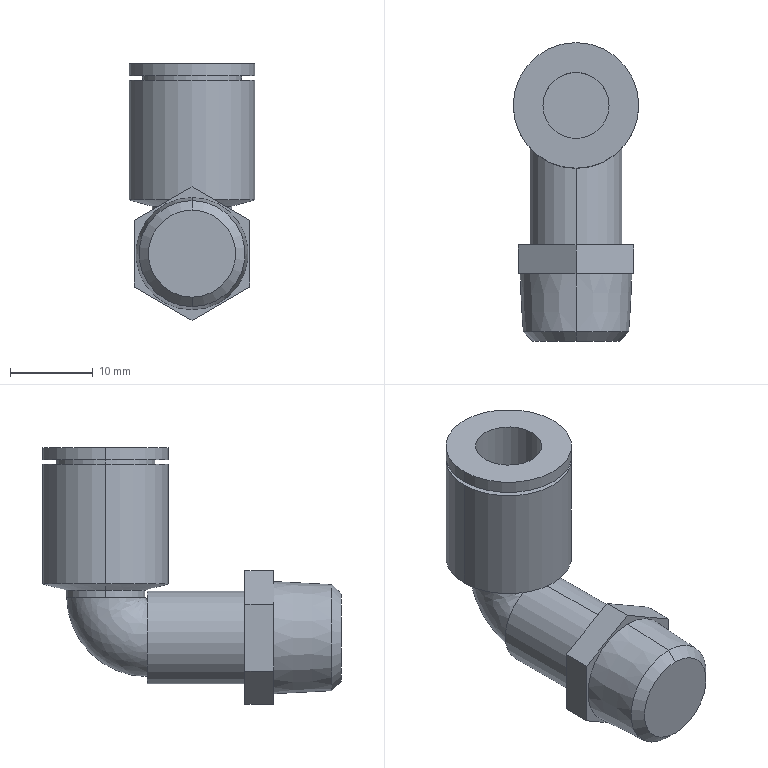Part | SolidWorks | features BaseBody 1 | 1 solid | 35 faces | box 15.2 x 36.1 x 31.083 mm | volume 5569 mm3 | plane 15 | cylinder 12 | cone 6 | spline 2 | commonest cylinder face diameters 15.2 x4 8 x2 9.637 x2 11.2 x2 12 x2
STEP:
#1=CARTESIAN_POINT('',(-7.6,28.5,21.));
#2=VERTEX_POINT('',#1);
#3=CARTESIAN_POINT('',(7.6,28.5,21.));
#4=VERTEX_POINT('',#3);
#5=CARTESIAN_POINT('',(0.,28.5,21.));
#6=DIRECTION('',(0.,0.,-1.));
#7=DIRECTION('',(-1.,0.,0.));
#8=AXIS2_PLACEMENT_3D('',#5,#6,#7);
#9=CIRCLE('',#8,7.6);
#10=EDGE_CURVE('',#2,#4,#9,.T.);
#11=ORIENTED_EDGE('',*,*,#10,.T.);
#12=CARTESIAN_POINT('',(7.6,28.5,6.495));
#13=VERTEX_POINT('',#12);
#14=CARTESIAN_POINT('',(7.6,28.5,13.748));
#15=DIRECTION('',(0.,0.,-1.));
#16=VECTOR('',#15,1000.);
#17=LINE('',#14,#16);
#18=EDGE_CURVE('',#4,#13,#17,.T.);
#19=ORIENTED_EDGE('',*,*,#18,.T.);
#20=CARTESIAN_POINT('',(-7.6,28.5,6.495));
#21=VERTEX_POINT('',#20);
#22=CARTESIAN_POINT('',(0.,28.5,6.495));
#23=DIRECTION('',(0.,0.,1.));
#24=DIRECTION('',(-1.,0.,0.));
#25=AXIS2_PLACEMENT_3D('',#22,#23,#24);
#26=CIRCLE('',#25,7.6);
#27=EDGE_CURVE('',#13,#21,#26,.T.);
#28=ORIENTED_EDGE('',*,*,#27,.T.);
#29=CARTESIAN_POINT('',(-7.6,28.5,13.748));
#30=DIRECTION('',(0.,0.,-1.));
#31=VECTOR('',#30,1000.);
#32=LINE('',#29,#31);
#33=EDGE_CURVE('',#2,#21,#32,.T.);
#34=ORIENTED_EDGE('',*,*,#33,.F.);
#35=EDGE_LOOP('',(#11,#19,#28,#34));
#36=FACE_OUTER_BOUND('',#35,.T.);
#37=CARTESIAN_POINT('',(0.,28.5,13.748));
#38=DIRECTION('',(0.,0.,-1.));
#39=DIRECTION('',(-1.,0.,0.));
#40=AXIS2_PLACEMENT_3D('',#37,#38,#39);
#41=CYLINDRICAL_SURFACE('',#40,7.6);
#42=ADVANCED_FACE('',(#36),#41,.T.);
#43=CARTESIAN_POINT('',(4.818,28.5,5.75));
#44=VERTEX_POINT('',#43);
#45=CARTESIAN_POINT('',(-4.818,28.5,5.75));
#46=VERTEX_POINT('',#45);
#47=CARTESIAN_POINT('',(0.,28.5,5.75));
#48=DIRECTION('',(0.,0.,1.));
#49=DIRECTION('',(-1.,0.,0.));
#50=AXIS2_PLACEMENT_3D('',#47,#48,#49);
#51=CIRCLE('',#50,4.818);
#52=EDGE_CURVE('',#44,#46,#51,.T.);
#53=ORIENTED_EDGE('',*,*,#52,.T.);
#54=CARTESIAN_POINT('',(-7.6,28.5,6.495));
#55=DIRECTION('',(-0.9659,0.,0.2588));
#56=VECTOR('',#55,1000.);
#57=LINE('',#54,#56);
#58=EDGE_CURVE('',#46,#21,#57,.T.);
#59=ORIENTED_EDGE('',*,*,#58,.T.);
#60=ORIENTED_EDGE('',*,*,#27,.F.);
#61=CARTESIAN_POINT('',(7.6,28.5,6.495));
#62=DIRECTION('',(0.9659,0.,0.2588));
#63=VECTOR('',#62,1000.);
#64=LINE('',#61,#63);
#65=EDGE_CURVE('',#44,#13,#64,.T.);
#66=ORIENTED_EDGE('',*,*,#65,.F.);
#67=EDGE_LOOP('',(#53,#59,#60,#66));
#68=FACE_OUTER_BOUND('',#67,.T.);
#69=CARTESIAN_POINT('',(0.,28.5,6.495));
#70=DIRECTION('',(0.,0.,1.));
#71=DIRECTION('',(1.,0.,0.));
#72=AXIS2_PLACEMENT_3D('',#69,#70,#71);
#73=CONICAL_SURFACE('',#72,7.6,1.309);
#74=ADVANCED_FACE('',(#68),#73,.T.);
#75=ORIENTED_EDGE('',*,*,#52,.F.);
#76=CARTESIAN_POINT('',(4.818,28.5,4.864));
#77=VERTEX_POINT('',#76);
#78=CARTESIAN_POINT('',(4.818,28.5,5.307));
#79=DIRECTION('',(0.,0.,-1.));
#80=VECTOR('',#79,1000.);
#81=LINE('',#78,#80);
#82=EDGE_CURVE('',#44,#77,#81,.T.);
#83=ORIENTED_EDGE('',*,*,#82,.T.);
#84=CARTESIAN_POINT('',(-4.818,28.5,4.864));
#85=VERTEX_POINT('',#84);
#86=CARTESIAN_POINT('',(0.,28.5,4.864));
#87=DIRECTION('',(0.,0.,1.));
#88=DIRECTION('',(-1.,0.,0.));
#89=AXIS2_PLACEMENT_3D('',#86,#87,#88);
#90=CIRCLE('',#89,4.818);
#91=EDGE_CURVE('',#77,#85,#90,.T.);
#92=ORIENTED_EDGE('',*,*,#91,.T.);
#93=CARTESIAN_POINT('',(-4.818,28.5,5.307));
#94=DIRECTION('',(0.,0.,-1.));
#95=VECTOR('',#94,1000.);
#96=LINE('',#93,#95);
#97=EDGE_CURVE('',#46,#85,#96,.T.);
#98=ORIENTED_EDGE('',*,*,#97,.F.);
#99=EDGE_LOOP('',(#75,#83,#92,#98));
#100=FACE_OUTER_BOUND('',#99,.T.);
#101=CARTESIAN_POINT('',(0.,28.5,5.307));
#102=DIRECTION('',(0.,0.,-1.));
#103=DIRECTION('',(-1.,0.,0.));
#104=AXIS2_PLACEMENT_3D('',#101,#102,#103);
#105=CYLINDRICAL_SURFACE('',#104,4.818);
#106=ADVANCED_FACE('',(#100),#105,.T.);
#107=CARTESIAN_POINT('',(-6.,28.5,21.5));
#108=VERTEX_POINT('',#107);
#109=CARTESIAN_POINT('',(6.,28.5,21.5));
#110=VERTEX_POINT('',#109);
#111=CARTESIAN_POINT('',(0.,28.5,21.5));
#112=DIRECTION('',(0.,0.,-1.));
#113=DIRECTION('',(-1.,0.,0.));
#114=AXIS2_PLACEMENT_3D('',#111,#112,#113);
#115=CIRCLE('',#114,6.);
#116=EDGE_CURVE('',#108,#110,#115,.T.);
#117=ORIENTED_EDGE('',*,*,#116,.T.);
#118=CARTESIAN_POINT('',(6.,28.5,21.));
#119=VERTEX_POINT('',#118);
#120=CARTESIAN_POINT('',(6.,28.5,21.25));
#121=DIRECTION('',(0.,0.,-1.));
#122=VECTOR('',#121,1000.);
#123=LINE('',#120,#122);
#124=EDGE_CURVE('',#110,#119,#123,.T.);
#125=ORIENTED_EDGE('',*,*,#124,.T.);
#126=CARTESIAN_POINT('',(-6.,28.5,21.));
#127=VERTEX_POINT('',#126);
#128=CARTESIAN_POINT('',(0.,28.5,21.));
#129=DIRECTION('',(0.,0.,-1.));
#130=DIRECTION('',(-1.,0.,0.));
#131=AXIS2_PLACEMENT_3D('',#128,#129,#130);
#132=CIRCLE('',#131,6.);
#133=EDGE_CURVE('',#127,#119,#132,.T.);
#134=ORIENTED_EDGE('',*,*,#133,.F.);
#135=CARTESIAN_POINT('',(-6.,28.5,21.25));
#136=DIRECTION('',(0.,0.,-1.));
#137=VECTOR('',#136,1000.);
#138=LINE('',#135,#137);
#139=EDGE_CURVE('',#108,#127,#138,.T.);
#140=ORIENTED_EDGE('',*,*,#139,.F.);
#141=EDGE_LOOP('',(#117,#125,#134,#140));
#142=FACE_OUTER_BOUND('',#141,.T.);
#143=CARTESIAN_POINT('',(0.,28.5,21.25));
#144=DIRECTION('',(0.,0.,-1.));
#145=DIRECTION('',(-1.,0.,0.));
#146=AXIS2_PLACEMENT_3D('',#143,#144,#145);
#147=CYLINDRICAL_SURFACE('',#146,6.);
#148=ADVANCED_FACE('',(#142),#147,.T.);
#149=CARTESIAN_POINT('',(0.,23.747,4.864));
#150=VERTEX_POINT('',#149);
#151=CARTESIAN_POINT('',(0.,33.211,4.864));
#152=VERTEX_POINT('',#151);
#153=CARTESIAN_POINT('',(0.,23.747,4.864));
#154=CARTESIAN_POINT('',(0.3117,23.747,4.864));
#155=CARTESIAN_POINT('',(0.6231,23.784,4.864));
#156=CARTESIAN_POINT('',(1.226,23.915,4.864));
#157=CARTESIAN_POINT('',(1.519,24.008,4.864));
#158=CARTESIAN_POINT('',(2.087,24.25,4.864));
#159=CARTESIAN_POINT('',(2.362,24.399,4.864));
#160=CARTESIAN_POINT('',(2.872,24.743,4.864));
#161=CARTESIAN_POINT('',(3.109,24.938,4.864));
#162=CARTESIAN_POINT('',(3.547,25.377,4.864));
#163=CARTESIAN_POINT('',(3.744,25.618,4.864));
#164=CARTESIAN_POINT('',(4.086,26.128,4.864));
#165=CARTESIAN_POINT('',(4.232,26.401,4.864));
#166=CARTESIAN_POINT('',(4.47,26.975,4.864));
#167=CARTESIAN_POINT('',(4.56,27.269,4.864));
#168=CARTESIAN_POINT('',(4.68,27.872,4.864));
#169=CARTESIAN_POINT('',(4.712,28.184,4.864));
#170=CARTESIAN_POINT('',(4.712,28.801,4.864));
#171=CARTESIAN_POINT('',(4.683,29.107,4.864));
#172=CARTESIAN_POINT('',(4.563,29.712,4.864));
#173=CARTESIAN_POINT('',(4.473,30.012,4.864));
#174=CARTESIAN_POINT('',(4.238,30.581,4.864));
#175=CARTESIAN_POINT('',(4.094,30.852,4.864));
#176=CARTESIAN_POINT('',(3.749,31.369,4.864));
#177=CARTESIAN_POINT('',(3.553,31.609,4.864));
#178=CARTESIAN_POINT('',(3.119,32.044,4.864));
#179=CARTESIAN_POINT('',(2.878,32.242,4.864));
#180=CARTESIAN_POINT('',(2.364,32.587,4.864));
#181=CARTESIAN_POINT('',(2.093,32.732,4.864));
#182=CARTESIAN_POINT('',(1.524,32.968,4.864));
#183=CARTESIAN_POINT('',(1.224,33.059,4.864));
#184=CARTESIAN_POINT('',(0.6186,33.18,4.864));
#185=CARTESIAN_POINT('',(0.3115,33.211,4.864));
#186=CARTESIAN_POINT('',(0.,33.211,4.864));
#187=B_SPLINE_CURVE_WITH_KNOTS('',3,(#153,#154,#155,#156,#157,#158,#159,#160,#161,#162,#163,#164,#165,#166,#167,#168,#169,#170,#171,#172,#173,#174,#175,#176,#177,#178,#179,#180,#181,#182,#183,#184,#185,#186),.UNSPECIFIED.,.F.,.F.,(4,2,2,2,2,2,2,2,2,2,2,2,2,2,2,2,4),(0.01474,0.01567,0.01659,0.01751,0.01843,0.01935,0.02027,0.02119,0.02211,0.02303,0.02396,0.02488,0.0258,0.02672,0.02764,0.02856,0.02948),.UNSPECIFIED.);
#188=EDGE_CURVE('',#150,#152,#187,.T.);
#189=ORIENTED_EDGE('',*,*,#188,.F.);
#190=CARTESIAN_POINT('',(0.,23.484,4.712));
#191=VERTEX_POINT('',#190);
#192=CARTESIAN_POINT('',(0.,23.484,5.016));
#193=DIRECTION('',(-1.,0.,0.));
#194=DIRECTION('',(0.,0.,1.));
#195=AXIS2_PLACEMENT_3D('',#192,#193,#194);
#196=CIRCLE('',#195,0.304);
#197=EDGE_CURVE('',#150,#191,#196,.T.);
#198=ORIENTED_EDGE('',*,*,#197,.T.);
#199=CARTESIAN_POINT('',(0.,23.484,-4.712));
#200=VERTEX_POINT('',#199);
#201=CARTESIAN_POINT('',(0.,23.484,4.712));
#202=CARTESIAN_POINT('',(0.3112,23.484,4.712));
#203=CARTESIAN_POINT('',(0.6228,23.484,4.681));
#204=CARTESIAN_POINT('',(1.227,23.484,4.56));
#205=CARTESIAN_POINT('',(1.521,23.484,4.47));
#206=CARTESIAN_POINT('',(2.09,23.484,4.234));
#207=CARTESIAN_POINT('',(2.366,23.484,4.086));
#208=CARTESIAN_POINT('',(2.877,23.484,3.744));
#209=CARTESIAN_POINT('',(3.114,23.484,3.55));
#210=CARTESIAN_POINT('',(3.553,23.484,3.111));
#211=CARTESIAN_POINT('',(3.749,23.484,2.871));
#212=CARTESIAN_POINT('',(4.09,23.484,2.361));
#213=CARTESIAN_POINT('',(4.236,23.484,2.086));
#214=CARTESIAN_POINT('',(4.473,23.484,1.514));
#215=CARTESIAN_POINT('',(4.562,23.484,1.22));
#216=CARTESIAN_POINT('',(4.682,23.484,0.617));
#217=CARTESIAN_POINT('',(4.712,23.484,0.3048));
#218=CARTESIAN_POINT('',(4.712,23.484,-0.3105));
#219=CARTESIAN_POINT('',(4.682,23.484,-0.6159));
#220=CARTESIAN_POINT('',(4.561,23.484,-1.222));
#221=CARTESIAN_POINT('',(4.47,23.484,-1.521));
#222=CARTESIAN_POINT('',(4.235,23.484,-2.088));
#223=CARTESIAN_POINT('',(4.09,23.484,-2.36));
#224=CARTESIAN_POINT('',(3.745,23.484,-2.877));
#225=CARTESIAN_POINT('',(3.55,23.484,-3.114));
#226=CARTESIAN_POINT('',(3.116,23.484,-3.548));
#227=CARTESIAN_POINT('',(2.874,23.484,-3.747));
#228=CARTESIAN_POINT('',(2.361,23.484,-4.09));
#229=CARTESIAN_POINT('',(2.09,23.484,-4.234));
#230=CARTESIAN_POINT('',(1.521,23.484,-4.47));
#231=CARTESIAN_POINT('',(1.221,23.484,-4.561));
#232=CARTESIAN_POINT('',(0.6176,23.484,-4.681));
#233=CARTESIAN_POINT('',(0.3112,23.484,-4.712));
#234=CARTESIAN_POINT('',(0.,23.484,-4.712));
#235=B_SPLINE_CURVE_WITH_KNOTS('',3,(#201,#202,#203,#204,#205,#206,#207,#208,#209,#210,#211,#212,#213,#214,#215,#216,#217,#218,#219,#220,#221,#222,#223,#224,#225,#226,#227,#228,#229,#230,#231,#232,#233,#234),.UNSPECIFIED.,.F.,.F.,(4,2,2,2,2,2,2,2,2,2,2,2,2,2,2,2,4),(0.007389,0.008313,0.009237,0.01016,0.01109,0.01201,0.01293,0.01386,0.01478,0.01571,0.01663,0.01755,0.01848,0.0194,0.02033,0.02125,0.02217),.UNSPECIFIED.);
#236=EDGE_CURVE('',#191,#200,#235,.T.);
#237=ORIENTED_EDGE('',*,*,#236,.T.);
#238=CARTESIAN_POINT('',(0.,23.484,5.016));
#239=DIRECTION('',(-1.,0.,0.));
#240=DIRECTION('',(0.,0.,1.));
#241=AXIS2_PLACEMENT_3D('',#238,#239,#240);
#242=CIRCLE('',#241,9.728);
#243=EDGE_CURVE('',#152,#200,#242,.T.);
#244=ORIENTED_EDGE('',*,*,#243,.F.);
#245=EDGE_LOOP('',(#189,#198,#237,#244));
#246=FACE_OUTER_BOUND('',#245,.T.);
#247=CARTESIAN_POINT('',(0.,33.212,4.955));
#248=CARTESIAN_POINT('',(0.,33.176,-0.7153));
#249=CARTESIAN_POINT('',(0.,29.154,-4.712));
#250=CARTESIAN_POINT('',(0.,23.484,-4.712));
#251=CARTESIAN_POINT('',(9.424,33.212,4.955));
#252=CARTESIAN_POINT('',(9.424,33.176,-0.7153));
#253=CARTESIAN_POINT('',(9.424,29.154,-4.712));
#254=CARTESIAN_POINT('',(9.424,23.484,-4.712));
#255=CARTESIAN_POINT('',(9.424,23.788,5.014));
#256=CARTESIAN_POINT('',(9.424,23.787,4.837));
#257=CARTESIAN_POINT('',(9.424,23.661,4.712));
#258=CARTESIAN_POINT('',(9.424,23.484,4.712));
#259=CARTESIAN_POINT('',(0.,23.788,5.014));
#260=CARTESIAN_POINT('',(0.,23.787,4.837));
#261=CARTESIAN_POINT('',(0.,23.661,4.712));
#262=CARTESIAN_POINT('',(0.,23.484,4.712));
#263=(BOUNDED_SURFACE()B_SPLINE_SURFACE(3,3,((#247,#248,#249,#250),(#251,#252,#253,#254),(#255,#256,#257,#258),(#259,#260,#261,#262)),.UNSPECIFIED.,.F.,.F.,.F.)B_SPLINE_SURFACE_WITH_KNOTS((4,4),(4,4),(0.,1.),(0.,1.),.UNSPECIFIED.)GEOMETRIC_REPRESENTATION_ITEM()RATIONAL_B_SPLINE_SURFACE(((1.,0.8062,0.8062,1.),(0.3333,0.2687,0.2687,0.3333),(0.3333,0.2687,0.2687,0.3333),(1.,0.8062,0.8062,1.)))REPRESENTATION_ITEM('')SURFACE());
#264=ADVANCED_FACE('',(#246),#263,.T.);
#265=CARTESIAN_POINT('',(-7.6,28.5,23.));
#266=VERTEX_POINT('',#265);
#267=CARTESIAN_POINT('',(7.6,28.5,23.));
#268=VERTEX_POINT('',#267);
#269=CARTESIAN_POINT('',(0.,28.5,23.));
#270=DIRECTION('',(0.,0.,-1.));
#271=DIRECTION('',(-1.,0.,0.));
#272=AXIS2_PLACEMENT_3D('',#269,#270,#271);
#273=CIRCLE('',#272,7.6);
#274=EDGE_CURVE('',#266,#268,#273,.T.);
#275=ORIENTED_EDGE('',*,*,#274,.T.);
#276=CARTESIAN_POINT('',(7.6,28.5,21.5));
#277=VERTEX_POINT('',#276);
#278=CARTESIAN_POINT('',(7.6,28.5,22.25));
#279=DIRECTION('',(0.,0.,-1.));
#280=VECTOR('',#279,1000.);
#281=LINE('',#278,#280);
#282=EDGE_CURVE('',#268,#277,#281,.T.);
#283=ORIENTED_EDGE('',*,*,#282,.T.);
#284=CARTESIAN_POINT('',(-7.6,28.5,21.5));
#285=VERTEX_POINT('',#284);
#286=CARTESIAN_POINT('',(0.,28.5,21.5));
#287=DIRECTION('',(0.,0.,-1.));
#288=DIRECTION('',(-1.,0.,0.));
#289=AXIS2_PLACEMENT_3D('',#286,#287,#288);
#290=CIRCLE('',#289,7.6);
#291=EDGE_CURVE('',#285,#277,#290,.T.);
#292=ORIENTED_EDGE('',*,*,#291,.F.);
#293=CARTESIAN_POINT('',(-7.6,28.5,22.25));
#294=DIRECTION('',(0.,0.,-1.));
#295=VECTOR('',#294,1000.);
#296=LINE('',#293,#295);
#297=EDGE_CURVE('',#266,#285,#296,.T.);
#298=ORIENTED_EDGE('',*,*,#297,.F.);
#299=EDGE_LOOP('',(#275,#283,#292,#298));
#300=FACE_OUTER_BOUND('',#299,.T.);
#301=CARTESIAN_POINT('',(0.,28.5,22.25));
#302=DIRECTION('',(0.,0.,-1.));
#303=DIRECTION('',(-1.,0.,0.));
#304=AXIS2_PLACEMENT_3D('',#301,#302,#303);
#305=CYLINDRICAL_SURFACE('',#304,7.6);
#306=ADVANCED_FACE('',(#300),#305,.T.);
#307=CARTESIAN_POINT('',(0.,11.66,5.6));
#308=VERTEX_POINT('',#307);
#309=CARTESIAN_POINT('',(0.,11.66,-5.6));
#310=VERTEX_POINT('',#309);
#311=CARTESIAN_POINT('',(0.,11.66,0.));
#312=DIRECTION('',(0.,1.,0.));
#313=DIRECTION('',(0.,0.,1.));
#314=AXIS2_PLACEMENT_3D('',#311,#312,#313);
#315=CIRCLE('',#314,5.6);
#316=EDGE_CURVE('',#308,#310,#315,.T.);
#317=ORIENTED_EDGE('',*,*,#316,.T.);
#318=CARTESIAN_POINT('',(0.,23.484,-5.6));
#319=VERTEX_POINT('',#318);
#320=CARTESIAN_POINT('',(0.,15.958,-5.6));
#321=DIRECTION('',(0.,1.,0.));
#322=VECTOR('',#321,1000.);
#323=LINE('',#320,#322);
#324=EDGE_CURVE('',#310,#319,#323,.T.);
#325=ORIENTED_EDGE('',*,*,#324,.T.);
#326=CARTESIAN_POINT('',(0.,23.484,5.6));
#327=VERTEX_POINT('',#326);
#328=CARTESIAN_POINT('',(0.,23.484,0.));
#329=DIRECTION('',(0.,1.,0.));
#330=DIRECTION('',(0.,0.,1.));
#331=AXIS2_PLACEMENT_3D('',#328,#329,#330);
#332=CIRCLE('',#331,5.6);
#333=EDGE_CURVE('',#327,#319,#332,.T.);
#334=ORIENTED_EDGE('',*,*,#333,.F.);
#335=CARTESIAN_POINT('',(0.,15.958,5.6));
#336=DIRECTION('',(0.,1.,0.));
#337=VECTOR('',#336,1000.);
#338=LINE('',#335,#337);
#339=EDGE_CURVE('',#308,#327,#338,.T.);
#340=ORIENTED_EDGE('',*,*,#339,.F.);
#341=EDGE_LOOP('',(#317,#325,#334,#340));
#342=FACE_OUTER_BOUND('',#341,.T.);
#343=CARTESIAN_POINT('',(0.,15.958,0.));
#344=DIRECTION('',(0.,1.,0.));
#345=DIRECTION('',(0.,0.,1.));
#346=AXIS2_PLACEMENT_3D('',#343,#344,#345);
#347=CYLINDRICAL_SURFACE('',#346,5.6);
#348=ADVANCED_FACE('',(#342),#347,.T.);
#349=CARTESIAN_POINT('',(-4.,28.5,4.5));
#350=VERTEX_POINT('',#349);
#351=CARTESIAN_POINT('',(4.,28.5,4.5));
#352=VERTEX_POINT('',#351);
#353=CARTESIAN_POINT('',(0.,28.5,4.5));
#354=DIRECTION('',(0.,0.,1.));
#355=DIRECTION('',(1.,0.,0.));
#356=AXIS2_PLACEMENT_3D('',#353,#354,#355);
#357=CIRCLE('',#356,4.);
#358=EDGE_CURVE('',#350,#352,#357,.T.);
#359=ORIENTED_EDGE('',*,*,#358,.F.);
#360=CARTESIAN_POINT('',(-4.,28.5,23.));
#361=VERTEX_POINT('',#360);
#362=CARTESIAN_POINT('',(-4.,28.5,41.5));
#363=DIRECTION('',(0.,0.,1.));
#364=VECTOR('',#363,1000.);
#365=LINE('',#362,#364);
#366=EDGE_CURVE('',#350,#361,#365,.T.);
#367=ORIENTED_EDGE('',*,*,#366,.T.);
#368=CARTESIAN_POINT('',(4.,28.5,23.));
#369=VERTEX_POINT('',#368);
#370=CARTESIAN_POINT('',(0.,28.5,23.));
#371=DIRECTION('',(0.,0.,-1.));
#372=DIRECTION('',(1.,0.,0.));
#373=AXIS2_PLACEMENT_3D('',#370,#371,#372);
#374=CIRCLE('',#373,4.);
#375=EDGE_CURVE('',#369,#361,#374,.T.);
#376=ORIENTED_EDGE('',*,*,#375,.F.);
#377=CARTESIAN_POINT('',(4.,28.5,41.5));
#378=DIRECTION('',(0.,0.,1.));
#379=VECTOR('',#378,1000.);
#380=LINE('',#377,#379);
#381=EDGE_CURVE('',#352,#369,#380,.T.);
#382=ORIENTED_EDGE('',*,*,#381,.F.);
#383=EDGE_LOOP('',(#359,#367,#376,#382));
#384=FACE_OUTER_BOUND('',#383,.T.);
#385=CARTESIAN_POINT('',(0.,28.5,41.5));
#386=DIRECTION('',(0.,0.,1.));
#387=DIRECTION('',(1.,0.,0.));
#388=AXIS2_PLACEMENT_3D('',#385,#386,#387);
#389=CYLINDRICAL_SURFACE('',#388,4.);
#390=ADVANCED_FACE('',(#384),#389,.F.);
#391=CARTESIAN_POINT('',(0.,1.146,6.418));
#392=VERTEX_POINT('',#391);
#393=CARTESIAN_POINT('',(0.,1.146,-6.418));
#394=VERTEX_POINT('',#393);
#395=CARTESIAN_POINT('',(0.,1.146,0.));
#396=DIRECTION('',(0.,1.,0.));
#397=DIRECTION('',(-1.,0.,0.));
#398=AXIS2_PLACEMENT_3D('',#395,#396,#397);
#399=CIRCLE('',#398,6.418);
#400=EDGE_CURVE('',#392,#394,#399,.T.);
#401=ORIENTED_EDGE('',*,*,#400,.T.);
#402=CARTESIAN_POINT('',(0.,8.16,-6.786));
#403=VERTEX_POINT('',#402);
#404=CARTESIAN_POINT('',(0.,8.16,-6.786));
#405=DIRECTION('',(0.,0.9986,-0.05234));
#406=VECTOR('',#405,1000.);
#407=LINE('',#404,#406);
#408=EDGE_CURVE('',#394,#403,#407,.T.);
#409=ORIENTED_EDGE('',*,*,#408,.T.);
#410=CARTESIAN_POINT('',(0.,8.16,6.786));
#411=VERTEX_POINT('',#410);
#412=CARTESIAN_POINT('',(0.,8.16,0.));
#413=DIRECTION('',(0.,-1.,0.));
#414=DIRECTION('',(0.,0.,1.));
#415=AXIS2_PLACEMENT_3D('',#412,#413,#414);
#416=CIRCLE('',#415,6.786);
#417=EDGE_CURVE('',#403,#411,#416,.T.);
#418=ORIENTED_EDGE('',*,*,#417,.T.);
#419=CARTESIAN_POINT('',(0.,8.16,6.786));
#420=DIRECTION('',(0.,0.9986,0.05234));
#421=VECTOR('',#420,1000.);
#422=LINE('',#419,#421);
#423=EDGE_CURVE('',#392,#411,#422,.T.);
#424=ORIENTED_EDGE('',*,*,#423,.F.);
#425=EDGE_LOOP('',(#401,#409,#418,#424));
#426=FACE_OUTER_BOUND('',#425,.T.);
#427=CARTESIAN_POINT('',(0.,8.16,0.));
#428=DIRECTION('',(0.,1.,0.));
#429=DIRECTION('',(0.,0.,1.));
#430=AXIS2_PLACEMENT_3D('',#427,#428,#429);
#431=CONICAL_SURFACE('',#430,6.786,0.05236);
#432=ADVANCED_FACE('',(#426),#431,.T.);
#433=CARTESIAN_POINT('',(0.,0.,5.272));
#434=VERTEX_POINT('',#433);
#435=CARTESIAN_POINT('',(0.,0.,-5.272));
#436=VERTEX_POINT('',#435);
#437=CARTESIAN_POINT('',(0.,0.,0.));
#438=DIRECTION('',(0.,1.,0.));
#439=DIRECTION('',(0.,0.,1.));
#440=AXIS2_PLACEMENT_3D('',#437,#438,#439);
#441=CIRCLE('',#440,5.272);
#442=EDGE_CURVE('',#434,#436,#441,.T.);
#443=ORIENTED_EDGE('',*,*,#442,.T.);
#444=CARTESIAN_POINT('',(0.,1.146,-6.418));
#445=DIRECTION('',(0.,0.7071,-0.7071));
#446=VECTOR('',#445,1000.);
#447=LINE('',#444,#446);
#448=EDGE_CURVE('',#436,#394,#447,.T.);
#449=ORIENTED_EDGE('',*,*,#448,.T.);
#450=ORIENTED_EDGE('',*,*,#400,.F.);
#451=CARTESIAN_POINT('',(0.,1.146,6.418));
#452=DIRECTION('',(0.,0.7071,0.7071));
#453=VECTOR('',#452,1000.);
#454=LINE('',#451,#453);
#455=EDGE_CURVE('',#434,#392,#454,.T.);
#456=ORIENTED_EDGE('',*,*,#455,.F.);
#457=EDGE_LOOP('',(#443,#449,#450,#456));
#458=FACE_OUTER_BOUND('',#457,.T.);
#459=CARTESIAN_POINT('',(0.,1.146,0.));
#460=DIRECTION('',(0.,1.,0.));
#461=DIRECTION('',(0.,0.,1.));
#462=AXIS2_PLACEMENT_3D('',#459,#460,#461);
#463=CONICAL_SURFACE('',#462,6.418,0.7854);
#464=ADVANCED_FACE('',(#458),#463,.T.);
#465=ORIENTED_EDGE('',*,*,#18,.F.);
#466=CARTESIAN_POINT('',(0.,28.5,21.));
#467=DIRECTION('',(0.,0.,-1.));
#468=DIRECTION('',(-1.,0.,0.));
#469=AXIS2_PLACEMENT_3D('',#466,#467,#468);
#470=CIRCLE('',#469,7.6);
#471=EDGE_CURVE('',#4,#2,#470,.T.);
#472=ORIENTED_EDGE('',*,*,#471,.T.);
#473=ORIENTED_EDGE('',*,*,#33,.T.);
#474=CARTESIAN_POINT('',(0.,28.5,6.495));
#475=DIRECTION('',(0.,0.,1.));
#476=DIRECTION('',(-1.,0.,0.));
#477=AXIS2_PLACEMENT_3D('',#474,#475,#476);
#478=CIRCLE('',#477,7.6);
#479=EDGE_CURVE('',#21,#13,#478,.T.);
#480=ORIENTED_EDGE('',*,*,#479,.T.);
#481=EDGE_LOOP('',(#465,#472,#473,#480));
#482=FACE_OUTER_BOUND('',#481,.T.);
#483=CARTESIAN_POINT('',(0.,28.5,13.748));
#484=DIRECTION('',(0.,0.,-1.));
#485=DIRECTION('',(-1.,0.,0.));
#486=AXIS2_PLACEMENT_3D('',#483,#484,#485);
#487=CYLINDRICAL_SURFACE('',#486,7.6);
#488=ADVANCED_FACE('',(#482),#487,.T.);
#489=ORIENTED_EDGE('',*,*,#58,.F.);
#490=CARTESIAN_POINT('',(0.,28.5,5.75));
#491=DIRECTION('',(0.,0.,1.));
#492=DIRECTION('',(-1.,0.,0.));
#493=AXIS2_PLACEMENT_3D('',#490,#491,#492);
#494=CIRCLE('',#493,4.818);
#495=EDGE_CURVE('',#46,#44,#494,.T.);
#496=ORIENTED_EDGE('',*,*,#495,.T.);
#497=ORIENTED_EDGE('',*,*,#65,.T.);
#498=ORIENTED_EDGE('',*,*,#479,.F.);
#499=EDGE_LOOP('',(#489,#496,#497,#498));
#500=FACE_OUTER_BOUND('',#499,.T.);
#501=CARTESIAN_POINT('',(0.,28.5,6.495));
#502=DIRECTION('',(0.,0.,1.));
#503=DIRECTION('',(1.,0.,0.));
#504=AXIS2_PLACEMENT_3D('',#501,#502,#503);
#505=CONICAL_SURFACE('',#504,7.6,1.309);
#506=ADVANCED_FACE('',(#500),#505,.T.);
#507=ORIENTED_EDGE('',*,*,#10,.F.);
#508=ORIENTED_EDGE('',*,*,#471,.F.);
#509=EDGE_LOOP('',(#507,#508));
#510=FACE_OUTER_BOUND('',#509,.T.);
#511=ORIENTED_EDGE('',*,*,#133,.T.);
#512=CARTESIAN_POINT('',(0.,28.5,21.));
#513=DIRECTION('',(0.,0.,-1.));
#514=DIRECTION('',(-1.,0.,0.));
#515=AXIS2_PLACEMENT_3D('',#512,#513,#514);
#516=CIRCLE('',#515,6.);
#517=EDGE_CURVE('',#119,#127,#516,.T.);
#518=ORIENTED_EDGE('',*,*,#517,.T.);
#519=EDGE_LOOP('',(#511,#518));
#520=FACE_BOUND('',#519,.T.);
#521=CARTESIAN_POINT('',(-6.8,28.5,21.));
#522=DIRECTION('',(0.,0.,1.));
#523=DIRECTION('',(1.,0.,0.));
#524=AXIS2_PLACEMENT_3D('',#521,#522,#523);
#525=PLANE('',#524);
#526=ADVANCED_FACE('',(#510,#520),#525,.T.);
#527=ORIENTED_EDGE('',*,*,#82,.F.);
#528=ORIENTED_EDGE('',*,*,#495,.F.);
#529=ORIENTED_EDGE('',*,*,#97,.T.);
#530=CARTESIAN_POINT('',(0.,28.5,4.864));
#531=DIRECTION('',(0.,0.,1.));
#532=DIRECTION('',(-1.,0.,0.));
#533=AXIS2_PLACEMENT_3D('',#530,#531,#532);
#534=CIRCLE('',#533,4.818);
#535=EDGE_CURVE('',#85,#77,#534,.T.);
#536=ORIENTED_EDGE('',*,*,#535,.T.);
#537=EDGE_LOOP('',(#527,#528,#529,#536));
#538=FACE_OUTER_BOUND('',#537,.T.);
#539=CARTESIAN_POINT('',(0.,28.5,5.307));
#540=DIRECTION('',(0.,0.,-1.));
#541=DIRECTION('',(-1.,0.,0.));
#542=AXIS2_PLACEMENT_3D('',#539,#540,#541);
#543=CYLINDRICAL_SURFACE('',#542,4.818);
#544=ADVANCED_FACE('',(#538),#543,.T.);
#545=ORIENTED_EDGE('',*,*,#124,.F.);
#546=CARTESIAN_POINT('',(0.,28.5,21.5));
#547=DIRECTION('',(0.,0.,-1.));
#548=DIRECTION('',(-1.,0.,0.));
#549=AXIS2_PLACEMENT_3D('',#546,#547,#548);
#550=CIRCLE('',#549,6.);
#551=EDGE_CURVE('',#110,#108,#550,.T.);
#552=ORIENTED_EDGE('',*,*,#551,.T.);
#553=ORIENTED_EDGE('',*,*,#139,.T.);
#554=ORIENTED_EDGE('',*,*,#517,.F.);
#555=EDGE_LOOP('',(#545,#552,#553,#554));
#556=FACE_OUTER_BOUND('',#555,.T.);
#557=CARTESIAN_POINT('',(0.,28.5,21.25));
#558=DIRECTION('',(0.,0.,-1.));
#559=DIRECTION('',(-1.,0.,0.));
#560=AXIS2_PLACEMENT_3D('',#557,#558,#559);
#561=CYLINDRICAL_SURFACE('',#560,6.);
#562=ADVANCED_FACE('',(#556),#561,.T.);
#563=CARTESIAN_POINT('',(0.,33.211,4.864));
#564=CARTESIAN_POINT('',(-0.3116,33.211,4.864));
#565=CARTESIAN_POINT('',(-0.618,33.18,4.864));
#566=CARTESIAN_POINT('',(-1.221,33.06,4.864));
#567=CARTESIAN_POINT('',(-1.52,32.97,4.864));
#568=CARTESIAN_POINT('',(-2.091,32.733,4.864));
#569=CARTESIAN_POINT('',(-2.362,32.588,4.864));
#570=CARTESIAN_POINT('',(-2.875,32.245,4.864));
#571=CARTESIAN_POINT('',(-3.117,32.046,4.864));
#572=CARTESIAN_POINT('',(-3.552,31.61,4.864));
#573=CARTESIAN_POINT('',(-3.747,31.372,4.864));
#574=CARTESIAN_POINT('',(-4.091,30.856,4.864));
#575=CARTESIAN_POINT('',(-4.237,30.582,4.864));
#576=CARTESIAN_POINT('',(-4.472,30.014,4.864));
#577=CARTESIAN_POINT('',(-4.562,29.717,4.864));
#578=CARTESIAN_POINT('',(-4.683,29.108,4.864));
#579=CARTESIAN_POINT('',(-4.712,28.802,4.864));
#580=CARTESIAN_POINT('',(-4.712,28.187,4.864));
#581=CARTESIAN_POINT('',(-4.681,27.874,4.864));
#582=CARTESIAN_POINT('',(-4.56,27.27,4.864));
#583=CARTESIAN_POINT('',(-4.47,26.976,4.864));
#584=CARTESIAN_POINT('',(-4.234,26.405,4.864));
#585=CARTESIAN_POINT('',(-4.086,26.129,4.864));
#586=CARTESIAN_POINT('',(-3.744,25.618,4.864));
#587=CARTESIAN_POINT('',(-3.549,25.379,4.864));
#588=CARTESIAN_POINT('',(-3.11,24.938,4.864));
#589=CARTESIAN_POINT('',(-2.871,24.743,4.864));
#590=CARTESIAN_POINT('',(-2.362,24.399,4.864));
#591=CARTESIAN_POINT('',(-2.087,24.25,4.864));
#592=CARTESIAN_POINT('',(-1.518,24.008,4.864));
#593=CARTESIAN_POINT('',(-1.225,23.914,4.864));
#594=CARTESIAN_POINT('',(-0.6232,23.784,4.864));
#595=CARTESIAN_POINT('',(-0.3118,23.747,4.864));
#596=CARTESIAN_POINT('',(0.,23.747,4.864));
#597=B_SPLINE_CURVE_WITH_KNOTS('',3,(#563,#564,#565,#566,#567,#568,#569,#570,#571,#572,#573,#574,#575,#576,#577,#578,#579,#580,#581,#582,#583,#584,#585,#586,#587,#588,#589,#590,#591,#592,#593,#594,#595,#596),.UNSPECIFIED.,.F.,.F.,(4,2,2,2,2,2,2,2,2,2,2,2,2,2,2,2,4),(0.,0.0009215,0.001843,0.002765,0.003686,0.004608,0.005529,0.006451,0.007372,0.008294,0.009215,0.01014,0.01106,0.01198,0.0129,0.01382,0.01474),.UNSPECIFIED.);
#598=EDGE_CURVE('',#152,#150,#597,.T.);
#599=ORIENTED_EDGE('',*,*,#598,.T.);
#600=ORIENTED_EDGE('',*,*,#188,.T.);
#601=EDGE_LOOP('',(#599,#600));
#602=FACE_BOUND('',#601,.T.);
#603=ORIENTED_EDGE('',*,*,#535,.F.);
#604=ORIENTED_EDGE('',*,*,#91,.F.);
#605=EDGE_LOOP('',(#603,#604));
#606=FACE_OUTER_BOUND('',#605,.T.);
#607=CARTESIAN_POINT('',(-2.409,28.5,4.864));
#608=DIRECTION('',(0.,0.,-1.));
#609=DIRECTION('',(-1.,0.,0.));
#610=AXIS2_PLACEMENT_3D('',#607,#608,#609);
#611=PLANE('',#610);
#612=ADVANCED_FACE('',(#602,#606),#611,.T.);
#613=ORIENTED_EDGE('',*,*,#116,.F.);
#614=ORIENTED_EDGE('',*,*,#551,.F.);
#615=EDGE_LOOP('',(#613,#614));
#616=FACE_BOUND('',#615,.T.);
#617=ORIENTED_EDGE('',*,*,#291,.T.);
#618=CARTESIAN_POINT('',(0.,28.5,21.5));
#619=DIRECTION('',(0.,0.,-1.));
#620=DIRECTION('',(-1.,0.,0.));
#621=AXIS2_PLACEMENT_3D('',#618,#619,#620);
#622=CIRCLE('',#621,7.6);
#623=EDGE_CURVE('',#277,#285,#622,.T.);
#624=ORIENTED_EDGE('',*,*,#623,.T.);
#625=EDGE_LOOP('',(#617,#624));
#626=FACE_OUTER_BOUND('',#625,.T.);
#627=CARTESIAN_POINT('',(-6.8,28.5,21.5));
#628=DIRECTION('',(0.,0.,-1.));
#629=DIRECTION('',(-1.,0.,0.));
#630=AXIS2_PLACEMENT_3D('',#627,#628,#629);
#631=PLANE('',#630);
#632=ADVANCED_FACE('',(#616,#626),#631,.T.);
#633=ORIENTED_EDGE('',*,*,#197,.F.);
#634=ORIENTED_EDGE('',*,*,#598,.F.);
#635=ORIENTED_EDGE('',*,*,#243,.T.);
#636=CARTESIAN_POINT('',(0.,23.484,-4.712));
#637=CARTESIAN_POINT('',(-0.3111,23.484,-4.712));
#638=CARTESIAN_POINT('',(-0.617,23.484,-4.681));
#639=CARTESIAN_POINT('',(-1.219,23.484,-4.562));
#640=CARTESIAN_POINT('',(-1.518,23.484,-4.472));
#641=CARTESIAN_POINT('',(-2.088,23.484,-4.235));
#642=CARTESIAN_POINT('',(-2.359,23.484,-4.091));
#643=CARTESIAN_POINT('',(-2.871,23.484,-3.749));
#644=CARTESIAN_POINT('',(-3.113,23.484,-3.551));
#645=CARTESIAN_POINT('',(-3.548,23.484,-3.116));
#646=CARTESIAN_POINT('',(-3.743,23.484,-2.879));
#647=CARTESIAN_POINT('',(-4.087,23.484,-2.365));
#648=CARTESIAN_POINT('',(-4.234,23.484,-2.091));
#649=CARTESIAN_POINT('',(-4.469,23.484,-1.525));
#650=CARTESIAN_POINT('',(-4.56,23.484,-1.228));
#651=CARTESIAN_POINT('',(-4.681,23.484,-0.6199));
#652=CARTESIAN_POINT('',(-4.712,23.484,-0.3122));
#653=CARTESIAN_POINT('',(-4.712,23.484,0.3099));
#654=CARTESIAN_POINT('',(-4.682,23.484,0.6167));
#655=CARTESIAN_POINT('',(-4.561,23.484,1.222));
#656=CARTESIAN_POINT('',(-4.47,23.484,1.521));
#657=CARTESIAN_POINT('',(-4.235,23.484,2.089));
#658=CARTESIAN_POINT('',(-4.09,23.484,2.36));
#659=CARTESIAN_POINT('',(-3.747,23.484,2.874));
#660=CARTESIAN_POINT('',(-3.549,23.484,3.115));
#661=CARTESIAN_POINT('',(-3.116,23.484,3.548));
#662=CARTESIAN_POINT('',(-2.876,23.484,3.745));
#663=CARTESIAN_POINT('',(-2.361,23.484,4.09));
#664=CARTESIAN_POINT('',(-2.09,23.484,4.234));
#665=CARTESIAN_POINT('',(-1.523,23.484,4.47));
#666=CARTESIAN_POINT('',(-1.224,23.484,4.561));
#667=CARTESIAN_POINT('',(-0.618,23.484,4.681));
#668=CARTESIAN_POINT('',(-0.3111,23.484,4.712));
#669=CARTESIAN_POINT('',(0.,23.484,4.712));
#670=B_SPLINE_CURVE_WITH_KNOTS('',3,(#636,#637,#638,#639,#640,#641,#642,#643,#644,#645,#646,#647,#648,#649,#650,#651,#652,#653,#654,#655,#656,#657,#658,#659,#660,#661,#662,#663,#664,#665,#666,#667,#668,#669),.UNSPECIFIED.,.F.,.F.,(4,2,2,2,2,2,2,2,2,2,2,2,2,2,2,2,4),(0.02217,0.0231,0.02402,0.02495,0.02587,0.02679,0.02772,0.02864,0.02956,0.03049,0.03141,0.03234,0.03326,0.03418,0.03511,0.03603,0.03695),.UNSPECIFIED.);
#671=EDGE_CURVE('',#200,#191,#670,.T.);
#672=ORIENTED_EDGE('',*,*,#671,.T.);
#673=EDGE_LOOP('',(#633,#634,#635,#672));
#674=FACE_OUTER_BOUND('',#673,.T.);
#675=CARTESIAN_POINT('',(0.,23.788,5.014));
#676=CARTESIAN_POINT('',(0.,23.787,4.837));
#677=CARTESIAN_POINT('',(0.,23.661,4.712));
#678=CARTESIAN_POINT('',(0.,23.484,4.712));
#679=CARTESIAN_POINT('',(-9.424,23.788,5.014));
#680=CARTESIAN_POINT('',(-9.424,23.787,4.837));
#681=CARTESIAN_POINT('',(-9.424,23.661,4.712));
#682=CARTESIAN_POINT('',(-9.424,23.484,4.712));
#683=CARTESIAN_POINT('',(-9.424,33.212,4.955));
#684=CARTESIAN_POINT('',(-9.424,33.176,-0.7153));
#685=CARTESIAN_POINT('',(-9.424,29.154,-4.712));
#686=CARTESIAN_POINT('',(-9.424,23.484,-4.712));
#687=CARTESIAN_POINT('',(0.,33.212,4.955));
#688=CARTESIAN_POINT('',(0.,33.176,-0.7153));
#689=CARTESIAN_POINT('',(0.,29.154,-4.712));
#690=CARTESIAN_POINT('',(0.,23.484,-4.712));
#691=(BOUNDED_SURFACE()B_SPLINE_SURFACE(3,3,((#675,#676,#677,#678),(#679,#680,#681,#682),(#683,#684,#685,#686),(#687,#688,#689,#690)),.UNSPECIFIED.,.F.,.F.,.F.)B_SPLINE_SURFACE_WITH_KNOTS((4,4),(4,4),(0.,1.),(0.,1.),.UNSPECIFIED.)GEOMETRIC_REPRESENTATION_ITEM()RATIONAL_B_SPLINE_SURFACE(((1.,0.8062,0.8062,1.),(0.3333,0.2687,0.2687,0.3333),(0.3333,0.2687,0.2687,0.3333),(1.,0.8062,0.8062,1.)))REPRESENTATION_ITEM('')SURFACE());
#692=ADVANCED_FACE('',(#674),#691,.T.);
#693=ORIENTED_EDGE('',*,*,#282,.F.);
#694=CARTESIAN_POINT('',(0.,28.5,23.));
#695=DIRECTION('',(0.,0.,-1.));
#696=DIRECTION('',(-1.,0.,0.));
#697=AXIS2_PLACEMENT_3D('',#694,#695,#696);
#698=CIRCLE('',#697,7.6);
#699=EDGE_CURVE('',#268,#266,#698,.T.);
#700=ORIENTED_EDGE('',*,*,#699,.T.);
#701=ORIENTED_EDGE('',*,*,#297,.T.);
#702=ORIENTED_EDGE('',*,*,#623,.F.);
#703=EDGE_LOOP('',(#693,#700,#701,#702));
#704=FACE_OUTER_BOUND('',#703,.T.);
#705=CARTESIAN_POINT('',(0.,28.5,22.25));
#706=DIRECTION('',(0.,0.,-1.));
#707=DIRECTION('',(-1.,0.,0.));
#708=AXIS2_PLACEMENT_3D('',#705,#706,#707);
#709=CYLINDRICAL_SURFACE('',#708,7.6);
#710=ADVANCED_FACE('',(#704),#709,.T.);
#711=ORIENTED_EDGE('',*,*,#333,.T.);
#712=CARTESIAN_POINT('',(0.,23.484,0.));
#713=DIRECTION('',(0.,1.,0.));
#714=DIRECTION('',(0.,0.,1.));
#715=AXIS2_PLACEMENT_3D('',#712,#713,#714);
#716=CIRCLE('',#715,5.6);
#717=EDGE_CURVE('',#319,#327,#716,.T.);
#718=ORIENTED_EDGE('',*,*,#717,.T.);
#719=EDGE_LOOP('',(#711,#718));
#720=FACE_OUTER_BOUND('',#719,.T.);
#721=ORIENTED_EDGE('',*,*,#671,.F.);
#722=ORIENTED_EDGE('',*,*,#236,.F.);
#723=EDGE_LOOP('',(#721,#722));
#724=FACE_BOUND('',#723,.T.);
#725=CARTESIAN_POINT('',(-2.8,23.484,0.));
#726=DIRECTION('',(0.,1.,0.));
#727=DIRECTION('',(0.,0.,1.));
#728=AXIS2_PLACEMENT_3D('',#725,#726,#727);
#729=PLANE('',#728);
#730=ADVANCED_FACE('',(#720,#724),#729,.T.);
#731=ORIENTED_EDGE('',*,*,#274,.F.);
#732=ORIENTED_EDGE('',*,*,#699,.F.);
#733=EDGE_LOOP('',(#731,#732));
#734=FACE_OUTER_BOUND('',#733,.T.);
#735=ORIENTED_EDGE('',*,*,#375,.T.);
#736=CARTESIAN_POINT('',(0.,28.5,23.));
#737=DIRECTION('',(0.,0.,-1.));
#738=DIRECTION('',(1.,0.,0.));
#739=AXIS2_PLACEMENT_3D('',#736,#737,#738);
#740=CIRCLE('',#739,4.);
#741=EDGE_CURVE('',#361,#369,#740,.T.);
#742=ORIENTED_EDGE('',*,*,#741,.T.);
#743=EDGE_LOOP('',(#735,#742));
#744=FACE_BOUND('',#743,.T.);
#745=CARTESIAN_POINT('',(-3.8,28.5,23.));
#746=DIRECTION('',(0.,0.,1.));
#747=DIRECTION('',(1.,0.,0.));
#748=AXIS2_PLACEMENT_3D('',#745,#746,#747);
#749=PLANE('',#748);
#750=ADVANCED_FACE('',(#734,#744),#749,.T.);
#751=ORIENTED_EDGE('',*,*,#324,.F.);
#752=CARTESIAN_POINT('',(0.,11.66,0.));
#753=DIRECTION('',(0.,1.,0.));
#754=DIRECTION('',(0.,0.,1.));
#755=AXIS2_PLACEMENT_3D('',#752,#753,#754);
#756=CIRCLE('',#755,5.6);
#757=EDGE_CURVE('',#310,#308,#756,.T.);
#758=ORIENTED_EDGE('',*,*,#757,.T.);
#759=ORIENTED_EDGE('',*,*,#339,.T.);
#760=ORIENTED_EDGE('',*,*,#717,.F.);
#761=EDGE_LOOP('',(#751,#758,#759,#760));
#762=FACE_OUTER_BOUND('',#761,.T.);
#763=CARTESIAN_POINT('',(0.,15.958,0.));
#764=DIRECTION('',(0.,1.,0.));
#765=DIRECTION('',(0.,0.,1.));
#766=AXIS2_PLACEMENT_3D('',#763,#764,#765);
#767=CYLINDRICAL_SURFACE('',#766,5.6);
#768=ADVANCED_FACE('',(#762),#767,.T.);
#769=ORIENTED_EDGE('',*,*,#366,.F.);
#770=CARTESIAN_POINT('',(0.,28.5,4.5));
#771=DIRECTION('',(0.,0.,1.));
#772=DIRECTION('',(1.,0.,0.));
#773=AXIS2_PLACEMENT_3D('',#770,#771,#772);
#774=CIRCLE('',#773,4.);
#775=EDGE_CURVE('',#352,#350,#774,.T.);
#776=ORIENTED_EDGE('',*,*,#775,.F.);
#777=ORIENTED_EDGE('',*,*,#381,.T.);
#778=ORIENTED_EDGE('',*,*,#741,.F.);
#779=EDGE_LOOP('',(#769,#776,#777,#778));
#780=FACE_OUTER_BOUND('',#779,.T.);
#781=CARTESIAN_POINT('',(0.,28.5,41.5));
#782=DIRECTION('',(0.,0.,1.));
#783=DIRECTION('',(1.,0.,0.));
#784=AXIS2_PLACEMENT_3D('',#781,#782,#783);
#785=CYLINDRICAL_SURFACE('',#784,4.);
#786=ADVANCED_FACE('',(#780),#785,.F.);
#787=ORIENTED_EDGE('',*,*,#316,.F.);
#788=ORIENTED_EDGE('',*,*,#757,.F.);
#789=EDGE_LOOP('',(#787,#788));
#790=FACE_BOUND('',#789,.T.);
#791=CARTESIAN_POINT('',(7.,11.66,4.041));
#792=VERTEX_POINT('',#791);
#793=CARTESIAN_POINT('',(7.,11.66,-4.041));
#794=VERTEX_POINT('',#793);
#795=CARTESIAN_POINT('',(7.,11.66,0.));
#796=DIRECTION('',(0.,0.,-1.));
#797=VECTOR('',#796,1000.);
#798=LINE('',#795,#797);
#799=EDGE_CURVE('',#792,#794,#798,.T.);
#800=ORIENTED_EDGE('',*,*,#799,.T.);
#801=CARTESIAN_POINT('',(0.,11.66,-8.083));
#802=VERTEX_POINT('',#801);
#803=CARTESIAN_POINT('',(7.,11.66,-4.041));
#804=DIRECTION('',(-0.866,0.,-0.5));
#805=VECTOR('',#804,1000.);
#806=LINE('',#803,#805);
#807=EDGE_CURVE('',#794,#802,#806,.T.);
#808=ORIENTED_EDGE('',*,*,#807,.T.);
#809=CARTESIAN_POINT('',(-7.,11.66,-4.041));
#810=VERTEX_POINT('',#809);
#811=CARTESIAN_POINT('',(0.,11.66,-8.083));
#812=DIRECTION('',(-0.866,0.,0.5));
#813=VECTOR('',#812,1000.);
#814=LINE('',#811,#813);
#815=EDGE_CURVE('',#802,#810,#814,.T.);
#816=ORIENTED_EDGE('',*,*,#815,.T.);
#817=CARTESIAN_POINT('',(-7.,11.66,4.041));
#818=VERTEX_POINT('',#817);
#819=CARTESIAN_POINT('',(-7.,11.66,0.));
#820=DIRECTION('',(0.,0.,1.));
#821=VECTOR('',#820,1000.);
#822=LINE('',#819,#821);
#823=EDGE_CURVE('',#810,#818,#822,.T.);
#824=ORIENTED_EDGE('',*,*,#823,.T.);
#825=CARTESIAN_POINT('',(0.,11.66,8.083));
#826=VERTEX_POINT('',#825);
#827=CARTESIAN_POINT('',(-7.,11.66,4.041));
#828=DIRECTION('',(0.866,0.,0.5));
#829=VECTOR('',#828,1000.);
#830=LINE('',#827,#829);
#831=EDGE_CURVE('',#818,#826,#830,.T.);
#832=ORIENTED_EDGE('',*,*,#831,.T.);
#833=CARTESIAN_POINT('',(0.,11.66,8.083));
#834=DIRECTION('',(0.866,0.,-0.5));
#835=VECTOR('',#834,1000.);
#836=LINE('',#833,#835);
#837=EDGE_CURVE('',#826,#792,#836,.T.);
#838=ORIENTED_EDGE('',*,*,#837,.T.);
#839=EDGE_LOOP('',(#800,#808,#816,#824,#832,#838));
#840=FACE_OUTER_BOUND('',#839,.T.);
#841=CARTESIAN_POINT('',(0.,11.66,0.));
#842=DIRECTION('',(0.,1.,0.));
#843=DIRECTION('',(0.,0.,1.));
#844=AXIS2_PLACEMENT_3D('',#841,#842,#843);
#845=PLANE('',#844);
#846=ADVANCED_FACE('',(#790,#840),#845,.T.);
#847=ORIENTED_EDGE('',*,*,#775,.T.);
#848=ORIENTED_EDGE('',*,*,#358,.T.);
#849=EDGE_LOOP('',(#847,#848));
#850=FACE_OUTER_BOUND('',#849,.T.);
#851=CARTESIAN_POINT('',(0.,28.5,4.5));
#852=DIRECTION('',(0.,0.,1.));
#853=DIRECTION('',(1.,0.,0.));
#854=AXIS2_PLACEMENT_3D('',#851,#852,#853);
#855=PLANE('',#854);
#856=ADVANCED_FACE('',(#850),#855,.T.);
#857=CARTESIAN_POINT('',(7.,8.16,-4.041));
#858=VERTEX_POINT('',#857);
#859=CARTESIAN_POINT('',(0.,8.16,-8.083));
#860=VERTEX_POINT('',#859);
#861=CARTESIAN_POINT('',(0.,8.16,-8.083));
#862=DIRECTION('',(-0.866,0.,-0.5));
#863=VECTOR('',#862,1000.);
#864=LINE('',#861,#863);
#865=EDGE_CURVE('',#858,#860,#864,.T.);
#866=ORIENTED_EDGE('',*,*,#865,.T.);
#867=CARTESIAN_POINT('',(0.,8.16,-8.083));
#868=DIRECTION('',(0.,1.,0.));
#869=VECTOR('',#868,1000.);
#870=LINE('',#867,#869);
#871=EDGE_CURVE('',#860,#802,#870,.T.);
#872=ORIENTED_EDGE('',*,*,#871,.T.);
#873=ORIENTED_EDGE('',*,*,#807,.F.);
#874=CARTESIAN_POINT('',(7.,8.16,-4.041));
#875=DIRECTION('',(0.,-1.,0.));
#876=VECTOR('',#875,1000.);
#877=LINE('',#874,#876);
#878=EDGE_CURVE('',#794,#858,#877,.T.);
#879=ORIENTED_EDGE('',*,*,#878,.T.);
#880=EDGE_LOOP('',(#866,#872,#873,#879));
#881=FACE_OUTER_BOUND('',#880,.T.);
#882=CARTESIAN_POINT('',(0.,8.16,-8.083));
#883=DIRECTION('',(0.5,0.,-0.866));
#884=DIRECTION('',(-0.866,0.,-0.5));
#885=AXIS2_PLACEMENT_3D('',#882,#883,#884);
#886=PLANE('',#885);
#887=ADVANCED_FACE('',(#881),#886,.T.);
#888=CARTESIAN_POINT('',(7.,8.16,4.041));
#889=VERTEX_POINT('',#888);
#890=CARTESIAN_POINT('',(7.,8.16,-4.041));
#891=DIRECTION('',(0.,0.,-1.));
#892=VECTOR('',#891,1000.);
#893=LINE('',#890,#892);
#894=EDGE_CURVE('',#889,#858,#893,.T.);
#895=ORIENTED_EDGE('',*,*,#894,.T.);
#896=ORIENTED_EDGE('',*,*,#878,.F.);
#897=ORIENTED_EDGE('',*,*,#799,.F.);
#898=CARTESIAN_POINT('',(7.,8.16,4.041));
#899=DIRECTION('',(0.,-1.,0.));
#900=VECTOR('',#899,1000.);
#901=LINE('',#898,#900);
#902=EDGE_CURVE('',#792,#889,#901,.T.);
#903=ORIENTED_EDGE('',*,*,#902,.T.);
#904=EDGE_LOOP('',(#895,#896,#897,#903));
#905=FACE_OUTER_BOUND('',#904,.T.);
#906=CARTESIAN_POINT('',(7.,8.16,-4.041));
#907=DIRECTION('',(1.,0.,0.));
#908=DIRECTION('',(0.,0.,-1.));
#909=AXIS2_PLACEMENT_3D('',#906,#907,#908);
#910=PLANE('',#909);
#911=ADVANCED_FACE('',(#905),#910,.T.);
#912=CARTESIAN_POINT('',(0.,8.16,8.083));
#913=VERTEX_POINT('',#912);
#914=CARTESIAN_POINT('',(7.,8.16,4.041));
#915=DIRECTION('',(0.866,0.,-0.5));
#916=VECTOR('',#915,1000.);
#917=LINE('',#914,#916);
#918=EDGE_CURVE('',#913,#889,#917,.T.);
#919=ORIENTED_EDGE('',*,*,#918,.T.);
#920=ORIENTED_EDGE('',*,*,#902,.F.);
#921=ORIENTED_EDGE('',*,*,#837,.F.);
#922=CARTESIAN_POINT('',(0.,8.16,8.083));
#923=DIRECTION('',(0.,-1.,0.));
#924=VECTOR('',#923,1000.);
#925=LINE('',#922,#924);
#926=EDGE_CURVE('',#826,#913,#925,.T.);
#927=ORIENTED_EDGE('',*,*,#926,.T.);
#928=EDGE_LOOP('',(#919,#920,#921,#927));
#929=FACE_OUTER_BOUND('',#928,.T.);
#930=CARTESIAN_POINT('',(7.,8.16,4.041));
#931=DIRECTION('',(0.5,0.,0.866));
#932=DIRECTION('',(0.866,0.,-0.5));
#933=AXIS2_PLACEMENT_3D('',#930,#931,#932);
#934=PLANE('',#933);
#935=ADVANCED_FACE('',(#929),#934,.T.);
#936=CARTESIAN_POINT('',(-7.,8.16,4.041));
#937=VERTEX_POINT('',#936);
#938=CARTESIAN_POINT('',(0.,8.16,8.083));
#939=DIRECTION('',(0.866,0.,0.5));
#940=VECTOR('',#939,1000.);
#941=LINE('',#938,#940);
#942=EDGE_CURVE('',#937,#913,#941,.T.);
#943=ORIENTED_EDGE('',*,*,#942,.T.);
#944=ORIENTED_EDGE('',*,*,#926,.F.);
#945=ORIENTED_EDGE('',*,*,#831,.F.);
#946=CARTESIAN_POINT('',(-7.,8.16,4.041));
#947=DIRECTION('',(0.,-1.,0.));
#948=VECTOR('',#947,1000.);
#949=LINE('',#946,#948);
#950=EDGE_CURVE('',#818,#937,#949,.T.);
#951=ORIENTED_EDGE('',*,*,#950,.T.);
#952=EDGE_LOOP('',(#943,#944,#945,#951));
#953=FACE_OUTER_BOUND('',#952,.T.);
#954=CARTESIAN_POINT('',(0.,8.16,8.083));
#955=DIRECTION('',(-0.5,0.,0.866));
#956=DIRECTION('',(0.866,0.,0.5));
#957=AXIS2_PLACEMENT_3D('',#954,#955,#956);
#958=PLANE('',#957);
#959=ADVANCED_FACE('',(#953),#958,.T.);
#960=CARTESIAN_POINT('',(-7.,8.16,-4.041));
#961=VERTEX_POINT('',#960);
#962=CARTESIAN_POINT('',(-7.,8.16,4.041));
#963=DIRECTION('',(0.,0.,1.));
#964=VECTOR('',#963,1000.);
#965=LINE('',#962,#964);
#966=EDGE_CURVE('',#961,#937,#965,.T.);
#967=ORIENTED_EDGE('',*,*,#966,.T.);
#968=ORIENTED_EDGE('',*,*,#950,.F.);
#969=ORIENTED_EDGE('',*,*,#823,.F.);
#970=CARTESIAN_POINT('',(-7.,8.16,-4.041));
#971=DIRECTION('',(0.,-1.,0.));
#972=VECTOR('',#971,1000.);
#973=LINE('',#970,#972);
#974=EDGE_CURVE('',#810,#961,#973,.T.);
#975=ORIENTED_EDGE('',*,*,#974,.T.);
#976=EDGE_LOOP('',(#967,#968,#969,#975));
#977=FACE_OUTER_BOUND('',#976,.T.);
#978=CARTESIAN_POINT('',(-7.,8.16,4.041));
#979=DIRECTION('',(-1.,0.,0.));
#980=DIRECTION('',(0.,0.,1.));
#981=AXIS2_PLACEMENT_3D('',#978,#979,#980);
#982=PLANE('',#981);
#983=ADVANCED_FACE('',(#977),#982,.T.);
#984=CARTESIAN_POINT('',(-7.,8.16,-4.041));
#985=DIRECTION('',(-0.866,0.,0.5));
#986=VECTOR('',#985,1000.);
#987=LINE('',#984,#986);
#988=EDGE_CURVE('',#860,#961,#987,.T.);
#989=ORIENTED_EDGE('',*,*,#988,.T.);
#990=ORIENTED_EDGE('',*,*,#974,.F.);
#991=ORIENTED_EDGE('',*,*,#815,.F.);
#992=ORIENTED_EDGE('',*,*,#871,.F.);
#993=EDGE_LOOP('',(#989,#990,#991,#992));
#994=FACE_OUTER_BOUND('',#993,.T.);
#995=CARTESIAN_POINT('',(-7.,8.16,-4.041));
#996=DIRECTION('',(-0.5,0.,-0.866));
#997=DIRECTION('',(-0.866,0.,0.5));
#998=AXIS2_PLACEMENT_3D('',#995,#996,#997);
#999=PLANE('',#998);
#1000=ADVANCED_FACE('',(#994),#999,.T.);
#1001=CARTESIAN_POINT('',(0.,8.16,0.));
#1002=DIRECTION('',(0.,-1.,0.));
#1003=DIRECTION('',(0.,0.,1.));
#1004=AXIS2_PLACEMENT_3D('',#1001,#1002,#1003);
#1005=CIRCLE('',#1004,6.786);
#1006=EDGE_CURVE('',#411,#403,#1005,.T.);
#1007=ORIENTED_EDGE('',*,*,#1006,.F.);
#1008=ORIENTED_EDGE('',*,*,#417,.F.);
#1009=EDGE_LOOP('',(#1007,#1008));
#1010=FACE_BOUND('',#1009,.T.);
#1011=ORIENTED_EDGE('',*,*,#988,.F.);
#1012=ORIENTED_EDGE('',*,*,#865,.F.);
#1013=ORIENTED_EDGE('',*,*,#894,.F.);
#1014=ORIENTED_EDGE('',*,*,#918,.F.);
#1015=ORIENTED_EDGE('',*,*,#942,.F.);
#1016=ORIENTED_EDGE('',*,*,#966,.F.);
#1017=EDGE_LOOP('',(#1011,#1012,#1013,#1014,#1015,#1016));
#1018=FACE_OUTER_BOUND('',#1017,.T.);
#1019=CARTESIAN_POINT('',(0.,8.16,0.));
#1020=DIRECTION('',(0.,1.,0.));
#1021=DIRECTION('',(0.,0.,1.));
#1022=AXIS2_PLACEMENT_3D('',#1019,#1020,#1021);
#1023=PLANE('',#1022);
#1024=ADVANCED_FACE('',(#1010,#1018),#1023,.F.);
#1025=ORIENTED_EDGE('',*,*,#408,.F.);
#1026=CARTESIAN_POINT('',(0.,1.146,0.));
#1027=DIRECTION('',(0.,1.,0.));
#1028=DIRECTION('',(-1.,0.,0.));
#1029=AXIS2_PLACEMENT_3D('',#1026,#1027,#1028);
#1030=CIRCLE('',#1029,6.418);
#1031=EDGE_CURVE('',#394,#392,#1030,.T.);
#1032=ORIENTED_EDGE('',*,*,#1031,.T.);
#1033=ORIENTED_EDGE('',*,*,#423,.T.);
#1034=ORIENTED_EDGE('',*,*,#1006,.T.);
#1035=EDGE_LOOP('',(#1025,#1032,#1033,#1034));
#1036=FACE_OUTER_BOUND('',#1035,.T.);
#1037=CARTESIAN_POINT('',(0.,8.16,0.));
#1038=DIRECTION('',(0.,1.,0.));
#1039=DIRECTION('',(0.,0.,1.));
#1040=AXIS2_PLACEMENT_3D('',#1037,#1038,#1039);
#1041=CONICAL_SURFACE('',#1040,6.786,0.05236);
#1042=ADVANCED_FACE('',(#1036),#1041,.T.);
#1043=ORIENTED_EDGE('',*,*,#448,.F.);
#1044=CARTESIAN_POINT('',(0.,0.,0.));
#1045=DIRECTION('',(0.,1.,0.));
#1046=DIRECTION('',(0.,0.,1.));
#1047=AXIS2_PLACEMENT_3D('',#1044,#1045,#1046);
#1048=CIRCLE('',#1047,5.272);
#1049=EDGE_CURVE('',#436,#434,#1048,.T.);
#1050=ORIENTED_EDGE('',*,*,#1049,.T.);
#1051=ORIENTED_EDGE('',*,*,#455,.T.);
#1052=ORIENTED_EDGE('',*,*,#1031,.F.);
#1053=EDGE_LOOP('',(#1043,#1050,#1051,#1052));
#1054=FACE_OUTER_BOUND('',#1053,.T.);
#1055=CARTESIAN_POINT('',(0.,1.146,0.));
#1056=DIRECTION('',(0.,1.,0.));
#1057=DIRECTION('',(0.,0.,1.));
#1058=AXIS2_PLACEMENT_3D('',#1055,#1056,#1057);
#1059=CONICAL_SURFACE('',#1058,6.418,0.7854);
#1060=ADVANCED_FACE('',(#1054),#1059,.T.);
#1061=ORIENTED_EDGE('',*,*,#442,.F.);
#1062=ORIENTED_EDGE('',*,*,#1049,.F.);
#1063=EDGE_LOOP('',(#1061,#1062));
#1064=FACE_OUTER_BOUND('',#1063,.T.);
#1065=CARTESIAN_POINT('',(-2.636,0.,0.));
#1066=DIRECTION('',(0.,-1.,0.));
#1067=DIRECTION('',(0.,0.,-1.));
#1068=AXIS2_PLACEMENT_3D('',#1065,#1066,#1067);
#1069=PLANE('',#1068);
#1070=ADVANCED_FACE('',(#1064),#1069,.T.);
#1071=CLOSED_SHELL('',(#42,#74,#106,#148,#264,#306,#348,#390,#432,#464,#488,#506,#526,#544,#562,#612,#632,#692,#710,#730,#750,#768,#786,#846,#856,#887,#911,#935,#959,#983,#1000,#1024,#1042,#1060,#1070));
#1072=MANIFOLD_SOLID_BREP('',#1071);
#1073=CARTESIAN_POINT('',(0.,0.,0.));
#1074=DIRECTION('',(0.,0.,1.));
#1075=DIRECTION('',(1.,0.,0.));
#1076=AXIS2_PLACEMENT_3D('',#1073,#1074,#1075);
#1077=(LENGTH_UNIT()NAMED_UNIT(*)SI_UNIT(.MILLI.,.METRE.));
#1078=UNCERTAINTY_MEASURE_WITH_UNIT(LENGTH_MEASURE(0.00001),#1077,'','');
#1079=(NAMED_UNIT(*)PLANE_ANGLE_UNIT()SI_UNIT($,.RADIAN.));
#1080=(NAMED_UNIT(*)SI_UNIT($,.STERADIAN.)SOLID_ANGLE_UNIT());
#1081=(GEOMETRIC_REPRESENTATION_CONTEXT(3)GLOBAL_UNCERTAINTY_ASSIGNED_CONTEXT((#1078))GLOBAL_UNIT_ASSIGNED_CONTEXT((#1077,#1079,#1080))REPRESENTATION_CONTEXT('',''));
#1082=ADVANCED_BREP_SHAPE_REPRESENTATION('',(#1072,#1076),#1081);